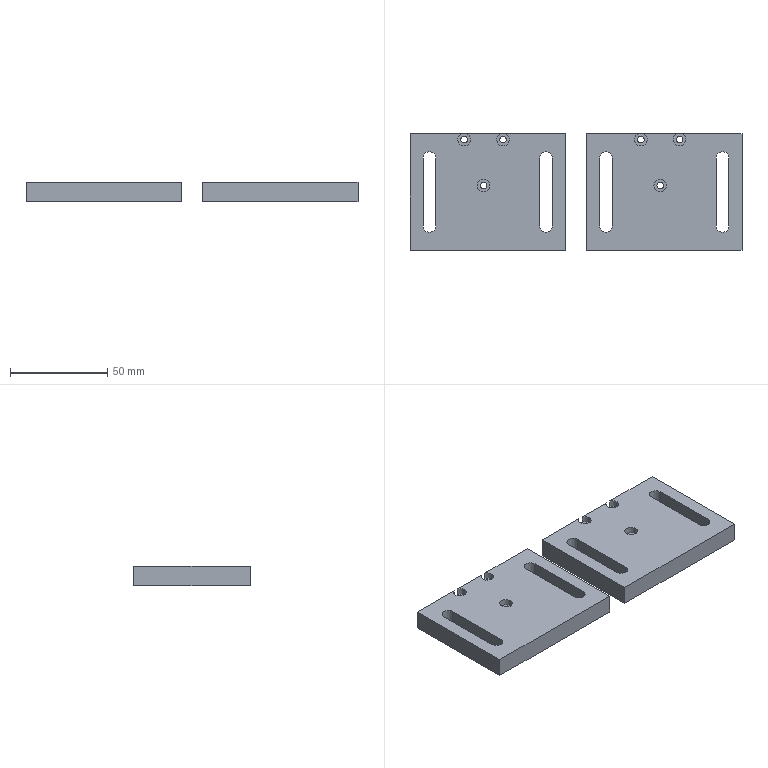Part | 2 solids | 46 faces | box 171 x 60 x 10 mm | volume 84542 mm3 | plane 26 | cylinder 20 | commonest cylinder face diameters 6.5 x14 3.4 x6
STEP:
#1=CARTESIAN_POINT('',(64.25,-17.5,0.));
#2=VERTEX_POINT('',#1);
#3=CARTESIAN_POINT('',(64.25,17.5,0.));
#4=VERTEX_POINT('',#3);
#5=CARTESIAN_POINT('',(64.25,-8.75,0.));
#6=DIRECTION('',(0.,1.,0.));
#7=VECTOR('',#6,1000.);
#8=LINE('',#5,#7);
#9=EDGE_CURVE('',#2,#4,#8,.T.);
#10=ORIENTED_EDGE('',*,*,#9,.T.);
#11=CARTESIAN_POINT('',(57.75,17.5,0.));
#12=VERTEX_POINT('',#11);
#13=CARTESIAN_POINT('',(61.,17.5,0.));
#14=DIRECTION('',(0.,0.,1.));
#15=DIRECTION('',(-1.,0.,0.));
#16=AXIS2_PLACEMENT_3D('',#13,#14,#15);
#17=CIRCLE('',#16,3.25);
#18=EDGE_CURVE('',#4,#12,#17,.T.);
#19=ORIENTED_EDGE('',*,*,#18,.T.);
#20=CARTESIAN_POINT('',(57.75,-17.5,0.));
#21=VERTEX_POINT('',#20);
#22=CARTESIAN_POINT('',(57.75,8.75,0.));
#23=DIRECTION('',(0.,-1.,0.));
#24=VECTOR('',#23,1000.);
#25=LINE('',#22,#24);
#26=EDGE_CURVE('',#12,#21,#25,.T.);
#27=ORIENTED_EDGE('',*,*,#26,.T.);
#28=CARTESIAN_POINT('',(61.,-17.5,0.));
#29=DIRECTION('',(0.,0.,1.));
#30=DIRECTION('',(1.,0.,0.));
#31=AXIS2_PLACEMENT_3D('',#28,#29,#30);
#32=CIRCLE('',#31,3.25);
#33=EDGE_CURVE('',#21,#2,#32,.T.);
#34=ORIENTED_EDGE('',*,*,#33,.T.);
#35=EDGE_LOOP('',(#10,#19,#27,#34));
#36=FACE_BOUND('',#35,.T.);
#37=CARTESIAN_POINT('',(124.25,-17.5,0.));
#38=VERTEX_POINT('',#37);
#39=CARTESIAN_POINT('',(124.25,17.5,0.));
#40=VERTEX_POINT('',#39);
#41=CARTESIAN_POINT('',(124.25,-8.75,0.));
#42=DIRECTION('',(0.,1.,0.));
#43=VECTOR('',#42,1000.);
#44=LINE('',#41,#43);
#45=EDGE_CURVE('',#38,#40,#44,.T.);
#46=ORIENTED_EDGE('',*,*,#45,.T.);
#47=CARTESIAN_POINT('',(117.75,17.5,0.));
#48=VERTEX_POINT('',#47);
#49=CARTESIAN_POINT('',(121.,17.5,0.));
#50=DIRECTION('',(0.,0.,1.));
#51=DIRECTION('',(-1.,0.,0.));
#52=AXIS2_PLACEMENT_3D('',#49,#50,#51);
#53=CIRCLE('',#52,3.25);
#54=EDGE_CURVE('',#40,#48,#53,.T.);
#55=ORIENTED_EDGE('',*,*,#54,.T.);
#56=CARTESIAN_POINT('',(117.75,-17.5,0.));
#57=VERTEX_POINT('',#56);
#58=CARTESIAN_POINT('',(117.75,8.75,0.));
#59=DIRECTION('',(0.,-1.,0.));
#60=VECTOR('',#59,1000.);
#61=LINE('',#58,#60);
#62=EDGE_CURVE('',#48,#57,#61,.T.);
#63=ORIENTED_EDGE('',*,*,#62,.T.);
#64=CARTESIAN_POINT('',(121.,-17.5,0.));
#65=DIRECTION('',(0.,0.,1.));
#66=DIRECTION('',(1.,0.,0.));
#67=AXIS2_PLACEMENT_3D('',#64,#65,#66);
#68=CIRCLE('',#67,3.25);
#69=EDGE_CURVE('',#57,#38,#68,.T.);
#70=ORIENTED_EDGE('',*,*,#69,.T.);
#71=EDGE_LOOP('',(#46,#55,#63,#70));
#72=FACE_BOUND('',#71,.T.);
#73=CARTESIAN_POINT('',(100.593,27.,0.));
#74=VERTEX_POINT('',#73);
#75=CARTESIAN_POINT('',(98.893,27.,0.));
#76=DIRECTION('',(0.,0.,1.));
#77=DIRECTION('',(1.,0.,0.));
#78=AXIS2_PLACEMENT_3D('',#75,#76,#77);
#79=CIRCLE('',#78,1.7);
#80=EDGE_CURVE('',#74,#74,#79,.T.);
#81=ORIENTED_EDGE('',*,*,#80,.T.);
#82=EDGE_LOOP('',(#81));
#83=FACE_BOUND('',#82,.T.);
#84=CARTESIAN_POINT('',(80.593,27.,0.));
#85=VERTEX_POINT('',#84);
#86=CARTESIAN_POINT('',(78.893,27.,0.));
#87=DIRECTION('',(0.,0.,1.));
#88=DIRECTION('',(1.,0.,0.));
#89=AXIS2_PLACEMENT_3D('',#86,#87,#88);
#90=CIRCLE('',#89,1.7);
#91=EDGE_CURVE('',#85,#85,#90,.T.);
#92=ORIENTED_EDGE('',*,*,#91,.T.);
#93=EDGE_LOOP('',(#92));
#94=FACE_BOUND('',#93,.T.);
#95=CARTESIAN_POINT('',(90.593,3.3,0.));
#96=VERTEX_POINT('',#95);
#97=CARTESIAN_POINT('',(88.893,3.3,0.));
#98=DIRECTION('',(0.,0.,1.));
#99=DIRECTION('',(1.,0.,0.));
#100=AXIS2_PLACEMENT_3D('',#97,#98,#99);
#101=CIRCLE('',#100,1.7);
#102=EDGE_CURVE('',#96,#96,#101,.T.);
#103=ORIENTED_EDGE('',*,*,#102,.T.);
#104=EDGE_LOOP('',(#103));
#105=FACE_BOUND('',#104,.T.);
#106=CARTESIAN_POINT('',(131.,-30.,0.));
#107=VERTEX_POINT('',#106);
#108=CARTESIAN_POINT('',(131.,30.,0.));
#109=VERTEX_POINT('',#108);
#110=CARTESIAN_POINT('',(131.,-30.,0.));
#111=DIRECTION('',(0.,1.,0.));
#112=VECTOR('',#111,1000.);
#113=LINE('',#110,#112);
#114=EDGE_CURVE('',#107,#109,#113,.T.);
#115=ORIENTED_EDGE('',*,*,#114,.F.);
#116=CARTESIAN_POINT('',(51.,-30.,0.));
#117=VERTEX_POINT('',#116);
#118=CARTESIAN_POINT('',(51.,-30.,0.));
#119=DIRECTION('',(1.,0.,0.));
#120=VECTOR('',#119,1000.);
#121=LINE('',#118,#120);
#122=EDGE_CURVE('',#117,#107,#121,.T.);
#123=ORIENTED_EDGE('',*,*,#122,.F.);
#124=CARTESIAN_POINT('',(51.,30.,0.));
#125=VERTEX_POINT('',#124);
#126=CARTESIAN_POINT('',(51.,30.,0.));
#127=DIRECTION('',(0.,-1.,0.));
#128=VECTOR('',#127,1000.);
#129=LINE('',#126,#128);
#130=EDGE_CURVE('',#125,#117,#129,.T.);
#131=ORIENTED_EDGE('',*,*,#130,.F.);
#132=CARTESIAN_POINT('',(131.,30.,0.));
#133=DIRECTION('',(-1.,0.,0.));
#134=VECTOR('',#133,1000.);
#135=LINE('',#132,#134);
#136=EDGE_CURVE('',#109,#125,#135,.T.);
#137=ORIENTED_EDGE('',*,*,#136,.F.);
#138=EDGE_LOOP('',(#115,#123,#131,#137));
#139=FACE_BOUND('',#138,.T.);
#140=CARTESIAN_POINT('',(91.,0.,0.));
#141=DIRECTION('',(0.,0.,1.));
#142=DIRECTION('',(1.,0.,0.));
#143=AXIS2_PLACEMENT_3D('',#140,#141,#142);
#144=PLANE('',#143);
#145=ADVANCED_FACE('',(#36,#72,#83,#94,#105,#139),#144,.F.);
#146=ORIENTED_EDGE('',*,*,#114,.T.);
#147=CARTESIAN_POINT('',(131.,30.,10.));
#148=VERTEX_POINT('',#147);
#149=CARTESIAN_POINT('',(131.,30.,0.));
#150=DIRECTION('',(0.,0.,1.));
#151=VECTOR('',#150,1000.);
#152=LINE('',#149,#151);
#153=EDGE_CURVE('',#109,#148,#152,.T.);
#154=ORIENTED_EDGE('',*,*,#153,.T.);
#155=CARTESIAN_POINT('',(131.,-30.,10.));
#156=VERTEX_POINT('',#155);
#157=CARTESIAN_POINT('',(131.,-30.,10.));
#158=DIRECTION('',(0.,1.,0.));
#159=VECTOR('',#158,1000.);
#160=LINE('',#157,#159);
#161=EDGE_CURVE('',#156,#148,#160,.T.);
#162=ORIENTED_EDGE('',*,*,#161,.F.);
#163=CARTESIAN_POINT('',(131.,-30.,0.));
#164=DIRECTION('',(0.,0.,1.));
#165=VECTOR('',#164,1000.);
#166=LINE('',#163,#165);
#167=EDGE_CURVE('',#107,#156,#166,.T.);
#168=ORIENTED_EDGE('',*,*,#167,.F.);
#169=EDGE_LOOP('',(#146,#154,#162,#168));
#170=FACE_BOUND('',#169,.T.);
#171=CARTESIAN_POINT('',(131.,-30.,0.));
#172=DIRECTION('',(1.,0.,0.));
#173=DIRECTION('',(0.,1.,0.));
#174=AXIS2_PLACEMENT_3D('',#171,#172,#173);
#175=PLANE('',#174);
#176=ADVANCED_FACE('',(#170),#175,.T.);
#177=CARTESIAN_POINT('',(80.143,30.,6.6));
#178=VERTEX_POINT('',#177);
#179=CARTESIAN_POINT('',(80.143,30.,10.));
#180=VERTEX_POINT('',#179);
#181=CARTESIAN_POINT('',(80.143,30.,8.3));
#182=DIRECTION('',(0.,0.,1.));
#183=VECTOR('',#182,1000.);
#184=LINE('',#181,#183);
#185=EDGE_CURVE('',#178,#180,#184,.T.);
#186=ORIENTED_EDGE('',*,*,#185,.T.);
#187=CARTESIAN_POINT('',(97.643,30.,10.));
#188=VERTEX_POINT('',#187);
#189=CARTESIAN_POINT('',(131.,30.,10.));
#190=DIRECTION('',(-1.,0.,0.));
#191=VECTOR('',#190,1000.);
#192=LINE('',#189,#191);
#193=EDGE_CURVE('',#188,#180,#192,.T.);
#194=ORIENTED_EDGE('',*,*,#193,.F.);
#195=CARTESIAN_POINT('',(97.643,30.,6.6));
#196=VERTEX_POINT('',#195);
#197=CARTESIAN_POINT('',(97.643,30.,8.3));
#198=DIRECTION('',(0.,0.,-1.));
#199=VECTOR('',#198,1000.);
#200=LINE('',#197,#199);
#201=EDGE_CURVE('',#188,#196,#200,.T.);
#202=ORIENTED_EDGE('',*,*,#201,.T.);
#203=CARTESIAN_POINT('',(100.143,30.,6.6));
#204=VERTEX_POINT('',#203);
#205=CARTESIAN_POINT('',(131.,30.,6.6));
#206=DIRECTION('',(1.,0.,0.));
#207=VECTOR('',#206,1000.);
#208=LINE('',#205,#207);
#209=EDGE_CURVE('',#196,#204,#208,.T.);
#210=ORIENTED_EDGE('',*,*,#209,.T.);
#211=CARTESIAN_POINT('',(100.143,30.,10.));
#212=VERTEX_POINT('',#211);
#213=CARTESIAN_POINT('',(100.143,30.,8.3));
#214=DIRECTION('',(0.,0.,1.));
#215=VECTOR('',#214,1000.);
#216=LINE('',#213,#215);
#217=EDGE_CURVE('',#204,#212,#216,.T.);
#218=ORIENTED_EDGE('',*,*,#217,.T.);
#219=CARTESIAN_POINT('',(131.,30.,10.));
#220=DIRECTION('',(-1.,0.,0.));
#221=VECTOR('',#220,1000.);
#222=LINE('',#219,#221);
#223=EDGE_CURVE('',#148,#212,#222,.T.);
#224=ORIENTED_EDGE('',*,*,#223,.F.);
#225=ORIENTED_EDGE('',*,*,#153,.F.);
#226=ORIENTED_EDGE('',*,*,#136,.T.);
#227=CARTESIAN_POINT('',(51.,30.,10.));
#228=VERTEX_POINT('',#227);
#229=CARTESIAN_POINT('',(51.,30.,0.));
#230=DIRECTION('',(0.,0.,1.));
#231=VECTOR('',#230,1000.);
#232=LINE('',#229,#231);
#233=EDGE_CURVE('',#125,#228,#232,.T.);
#234=ORIENTED_EDGE('',*,*,#233,.T.);
#235=CARTESIAN_POINT('',(77.643,30.,10.));
#236=VERTEX_POINT('',#235);
#237=CARTESIAN_POINT('',(131.,30.,10.));
#238=DIRECTION('',(-1.,0.,0.));
#239=VECTOR('',#238,1000.);
#240=LINE('',#237,#239);
#241=EDGE_CURVE('',#236,#228,#240,.T.);
#242=ORIENTED_EDGE('',*,*,#241,.F.);
#243=CARTESIAN_POINT('',(77.643,30.,6.6));
#244=VERTEX_POINT('',#243);
#245=CARTESIAN_POINT('',(77.643,30.,8.3));
#246=DIRECTION('',(0.,0.,-1.));
#247=VECTOR('',#246,1000.);
#248=LINE('',#245,#247);
#249=EDGE_CURVE('',#236,#244,#248,.T.);
#250=ORIENTED_EDGE('',*,*,#249,.T.);
#251=CARTESIAN_POINT('',(131.,30.,6.6));
#252=DIRECTION('',(1.,0.,0.));
#253=VECTOR('',#252,1000.);
#254=LINE('',#251,#253);
#255=EDGE_CURVE('',#244,#178,#254,.T.);
#256=ORIENTED_EDGE('',*,*,#255,.T.);
#257=EDGE_LOOP('',(#186,#194,#202,#210,#218,#224,#225,#226,#234,#242,#250,#256));
#258=FACE_BOUND('',#257,.T.);
#259=CARTESIAN_POINT('',(131.,30.,0.));
#260=DIRECTION('',(0.,1.,0.));
#261=DIRECTION('',(-1.,0.,0.));
#262=AXIS2_PLACEMENT_3D('',#259,#260,#261);
#263=PLANE('',#262);
#264=ADVANCED_FACE('',(#258),#263,.T.);
#265=ORIENTED_EDGE('',*,*,#130,.T.);
#266=CARTESIAN_POINT('',(51.,-30.,10.));
#267=VERTEX_POINT('',#266);
#268=CARTESIAN_POINT('',(51.,-30.,0.));
#269=DIRECTION('',(0.,0.,1.));
#270=VECTOR('',#269,1000.);
#271=LINE('',#268,#270);
#272=EDGE_CURVE('',#117,#267,#271,.T.);
#273=ORIENTED_EDGE('',*,*,#272,.T.);
#274=CARTESIAN_POINT('',(51.,30.,10.));
#275=DIRECTION('',(0.,-1.,0.));
#276=VECTOR('',#275,1000.);
#277=LINE('',#274,#276);
#278=EDGE_CURVE('',#228,#267,#277,.T.);
#279=ORIENTED_EDGE('',*,*,#278,.F.);
#280=ORIENTED_EDGE('',*,*,#233,.F.);
#281=EDGE_LOOP('',(#265,#273,#279,#280));
#282=FACE_BOUND('',#281,.T.);
#283=CARTESIAN_POINT('',(51.,30.,0.));
#284=DIRECTION('',(-1.,0.,0.));
#285=DIRECTION('',(0.,-1.,0.));
#286=AXIS2_PLACEMENT_3D('',#283,#284,#285);
#287=PLANE('',#286);
#288=ADVANCED_FACE('',(#282),#287,.T.);
#289=ORIENTED_EDGE('',*,*,#122,.T.);
#290=ORIENTED_EDGE('',*,*,#167,.T.);
#291=CARTESIAN_POINT('',(51.,-30.,10.));
#292=DIRECTION('',(1.,0.,0.));
#293=VECTOR('',#292,1000.);
#294=LINE('',#291,#293);
#295=EDGE_CURVE('',#267,#156,#294,.T.);
#296=ORIENTED_EDGE('',*,*,#295,.F.);
#297=ORIENTED_EDGE('',*,*,#272,.F.);
#298=EDGE_LOOP('',(#289,#290,#296,#297));
#299=FACE_BOUND('',#298,.T.);
#300=CARTESIAN_POINT('',(51.,-30.,0.));
#301=DIRECTION('',(0.,-1.,0.));
#302=DIRECTION('',(1.,0.,0.));
#303=AXIS2_PLACEMENT_3D('',#300,#301,#302);
#304=PLANE('',#303);
#305=ADVANCED_FACE('',(#299),#304,.T.);
#306=CARTESIAN_POINT('',(64.25,-17.5,10.));
#307=VERTEX_POINT('',#306);
#308=CARTESIAN_POINT('',(57.75,-17.5,10.));
#309=VERTEX_POINT('',#308);
#310=CARTESIAN_POINT('',(61.,-17.5,10.));
#311=DIRECTION('',(0.,0.,-1.));
#312=DIRECTION('',(1.,0.,0.));
#313=AXIS2_PLACEMENT_3D('',#310,#311,#312);
#314=CIRCLE('',#313,3.25);
#315=EDGE_CURVE('',#307,#309,#314,.T.);
#316=ORIENTED_EDGE('',*,*,#315,.F.);
#317=CARTESIAN_POINT('',(64.25,-17.5,0.));
#318=DIRECTION('',(0.,0.,1.));
#319=VECTOR('',#318,1000.);
#320=LINE('',#317,#319);
#321=EDGE_CURVE('',#2,#307,#320,.T.);
#322=ORIENTED_EDGE('',*,*,#321,.F.);
#323=ORIENTED_EDGE('',*,*,#33,.F.);
#324=CARTESIAN_POINT('',(57.75,-17.5,0.));
#325=DIRECTION('',(0.,0.,1.));
#326=VECTOR('',#325,1000.);
#327=LINE('',#324,#326);
#328=EDGE_CURVE('',#21,#309,#327,.T.);
#329=ORIENTED_EDGE('',*,*,#328,.T.);
#330=EDGE_LOOP('',(#316,#322,#323,#329));
#331=FACE_BOUND('',#330,.T.);
#332=CARTESIAN_POINT('',(61.,-17.5,0.));
#333=DIRECTION('',(0.,0.,1.));
#334=DIRECTION('',(1.,0.,0.));
#335=AXIS2_PLACEMENT_3D('',#332,#333,#334);
#336=CYLINDRICAL_SURFACE('',#335,3.25);
#337=ADVANCED_FACE('',(#331),#336,.F.);
#338=CARTESIAN_POINT('',(64.25,17.5,10.));
#339=VERTEX_POINT('',#338);
#340=CARTESIAN_POINT('',(64.25,-8.75,10.));
#341=DIRECTION('',(0.,-1.,0.));
#342=VECTOR('',#341,1000.);
#343=LINE('',#340,#342);
#344=EDGE_CURVE('',#339,#307,#343,.T.);
#345=ORIENTED_EDGE('',*,*,#344,.F.);
#346=CARTESIAN_POINT('',(64.25,17.5,0.));
#347=DIRECTION('',(0.,0.,1.));
#348=VECTOR('',#347,1000.);
#349=LINE('',#346,#348);
#350=EDGE_CURVE('',#4,#339,#349,.T.);
#351=ORIENTED_EDGE('',*,*,#350,.F.);
#352=ORIENTED_EDGE('',*,*,#9,.F.);
#353=ORIENTED_EDGE('',*,*,#321,.T.);
#354=EDGE_LOOP('',(#345,#351,#352,#353));
#355=FACE_BOUND('',#354,.T.);
#356=CARTESIAN_POINT('',(64.25,-17.5,0.));
#357=DIRECTION('',(1.,0.,0.));
#358=DIRECTION('',(0.,1.,0.));
#359=AXIS2_PLACEMENT_3D('',#356,#357,#358);
#360=PLANE('',#359);
#361=ADVANCED_FACE('',(#355),#360,.F.);
#362=CARTESIAN_POINT('',(57.75,17.5,10.));
#363=VERTEX_POINT('',#362);
#364=CARTESIAN_POINT('',(61.,17.5,10.));
#365=DIRECTION('',(0.,0.,-1.));
#366=DIRECTION('',(-1.,0.,0.));
#367=AXIS2_PLACEMENT_3D('',#364,#365,#366);
#368=CIRCLE('',#367,3.25);
#369=EDGE_CURVE('',#363,#339,#368,.T.);
#370=ORIENTED_EDGE('',*,*,#369,.F.);
#371=CARTESIAN_POINT('',(57.75,17.5,0.));
#372=DIRECTION('',(0.,0.,1.));
#373=VECTOR('',#372,1000.);
#374=LINE('',#371,#373);
#375=EDGE_CURVE('',#12,#363,#374,.T.);
#376=ORIENTED_EDGE('',*,*,#375,.F.);
#377=ORIENTED_EDGE('',*,*,#18,.F.);
#378=ORIENTED_EDGE('',*,*,#350,.T.);
#379=EDGE_LOOP('',(#370,#376,#377,#378));
#380=FACE_BOUND('',#379,.T.);
#381=CARTESIAN_POINT('',(61.,17.5,0.));
#382=DIRECTION('',(0.,0.,1.));
#383=DIRECTION('',(-1.,0.,0.));
#384=AXIS2_PLACEMENT_3D('',#381,#382,#383);
#385=CYLINDRICAL_SURFACE('',#384,3.25);
#386=ADVANCED_FACE('',(#380),#385,.F.);
#387=CARTESIAN_POINT('',(57.75,8.75,10.));
#388=DIRECTION('',(0.,1.,0.));
#389=VECTOR('',#388,1000.);
#390=LINE('',#387,#389);
#391=EDGE_CURVE('',#309,#363,#390,.T.);
#392=ORIENTED_EDGE('',*,*,#391,.F.);
#393=ORIENTED_EDGE('',*,*,#328,.F.);
#394=ORIENTED_EDGE('',*,*,#26,.F.);
#395=ORIENTED_EDGE('',*,*,#375,.T.);
#396=EDGE_LOOP('',(#392,#393,#394,#395));
#397=FACE_BOUND('',#396,.T.);
#398=CARTESIAN_POINT('',(57.75,17.5,0.));
#399=DIRECTION('',(-1.,0.,0.));
#400=DIRECTION('',(0.,-1.,0.));
#401=AXIS2_PLACEMENT_3D('',#398,#399,#400);
#402=PLANE('',#401);
#403=ADVANCED_FACE('',(#397),#402,.F.);
#404=CARTESIAN_POINT('',(124.25,-17.5,10.));
#405=VERTEX_POINT('',#404);
#406=CARTESIAN_POINT('',(117.75,-17.5,10.));
#407=VERTEX_POINT('',#406);
#408=CARTESIAN_POINT('',(121.,-17.5,10.));
#409=DIRECTION('',(0.,0.,-1.));
#410=DIRECTION('',(1.,0.,0.));
#411=AXIS2_PLACEMENT_3D('',#408,#409,#410);
#412=CIRCLE('',#411,3.25);
#413=EDGE_CURVE('',#405,#407,#412,.T.);
#414=ORIENTED_EDGE('',*,*,#413,.F.);
#415=CARTESIAN_POINT('',(124.25,-17.5,0.));
#416=DIRECTION('',(0.,0.,1.));
#417=VECTOR('',#416,1000.);
#418=LINE('',#415,#417);
#419=EDGE_CURVE('',#38,#405,#418,.T.);
#420=ORIENTED_EDGE('',*,*,#419,.F.);
#421=ORIENTED_EDGE('',*,*,#69,.F.);
#422=CARTESIAN_POINT('',(117.75,-17.5,0.));
#423=DIRECTION('',(0.,0.,1.));
#424=VECTOR('',#423,1000.);
#425=LINE('',#422,#424);
#426=EDGE_CURVE('',#57,#407,#425,.T.);
#427=ORIENTED_EDGE('',*,*,#426,.T.);
#428=EDGE_LOOP('',(#414,#420,#421,#427));
#429=FACE_BOUND('',#428,.T.);
#430=CARTESIAN_POINT('',(121.,-17.5,0.));
#431=DIRECTION('',(0.,0.,1.));
#432=DIRECTION('',(1.,0.,0.));
#433=AXIS2_PLACEMENT_3D('',#430,#431,#432);
#434=CYLINDRICAL_SURFACE('',#433,3.25);
#435=ADVANCED_FACE('',(#429),#434,.F.);
#436=CARTESIAN_POINT('',(124.25,17.5,10.));
#437=VERTEX_POINT('',#436);
#438=CARTESIAN_POINT('',(124.25,-8.75,10.));
#439=DIRECTION('',(0.,-1.,0.));
#440=VECTOR('',#439,1000.);
#441=LINE('',#438,#440);
#442=EDGE_CURVE('',#437,#405,#441,.T.);
#443=ORIENTED_EDGE('',*,*,#442,.F.);
#444=CARTESIAN_POINT('',(124.25,17.5,0.));
#445=DIRECTION('',(0.,0.,1.));
#446=VECTOR('',#445,1000.);
#447=LINE('',#444,#446);
#448=EDGE_CURVE('',#40,#437,#447,.T.);
#449=ORIENTED_EDGE('',*,*,#448,.F.);
#450=ORIENTED_EDGE('',*,*,#45,.F.);
#451=ORIENTED_EDGE('',*,*,#419,.T.);
#452=EDGE_LOOP('',(#443,#449,#450,#451));
#453=FACE_BOUND('',#452,.T.);
#454=CARTESIAN_POINT('',(124.25,-17.5,0.));
#455=DIRECTION('',(1.,0.,0.));
#456=DIRECTION('',(0.,1.,0.));
#457=AXIS2_PLACEMENT_3D('',#454,#455,#456);
#458=PLANE('',#457);
#459=ADVANCED_FACE('',(#453),#458,.F.);
#460=CARTESIAN_POINT('',(117.75,17.5,10.));
#461=VERTEX_POINT('',#460);
#462=CARTESIAN_POINT('',(121.,17.5,10.));
#463=DIRECTION('',(0.,0.,-1.));
#464=DIRECTION('',(-1.,0.,0.));
#465=AXIS2_PLACEMENT_3D('',#462,#463,#464);
#466=CIRCLE('',#465,3.25);
#467=EDGE_CURVE('',#461,#437,#466,.T.);
#468=ORIENTED_EDGE('',*,*,#467,.F.);
#469=CARTESIAN_POINT('',(117.75,17.5,0.));
#470=DIRECTION('',(0.,0.,1.));
#471=VECTOR('',#470,1000.);
#472=LINE('',#469,#471);
#473=EDGE_CURVE('',#48,#461,#472,.T.);
#474=ORIENTED_EDGE('',*,*,#473,.F.);
#475=ORIENTED_EDGE('',*,*,#54,.F.);
#476=ORIENTED_EDGE('',*,*,#448,.T.);
#477=EDGE_LOOP('',(#468,#474,#475,#476));
#478=FACE_BOUND('',#477,.T.);
#479=CARTESIAN_POINT('',(121.,17.5,0.));
#480=DIRECTION('',(0.,0.,1.));
#481=DIRECTION('',(-1.,0.,0.));
#482=AXIS2_PLACEMENT_3D('',#479,#480,#481);
#483=CYLINDRICAL_SURFACE('',#482,3.25);
#484=ADVANCED_FACE('',(#478),#483,.F.);
#485=CARTESIAN_POINT('',(117.75,8.75,10.));
#486=DIRECTION('',(0.,1.,0.));
#487=VECTOR('',#486,1000.);
#488=LINE('',#485,#487);
#489=EDGE_CURVE('',#407,#461,#488,.T.);
#490=ORIENTED_EDGE('',*,*,#489,.F.);
#491=ORIENTED_EDGE('',*,*,#426,.F.);
#492=ORIENTED_EDGE('',*,*,#62,.F.);
#493=ORIENTED_EDGE('',*,*,#473,.T.);
#494=EDGE_LOOP('',(#490,#491,#492,#493));
#495=FACE_BOUND('',#494,.T.);
#496=CARTESIAN_POINT('',(117.75,17.5,0.));
#497=DIRECTION('',(-1.,0.,0.));
#498=DIRECTION('',(0.,-1.,0.));
#499=AXIS2_PLACEMENT_3D('',#496,#497,#498);
#500=PLANE('',#499);
#501=ADVANCED_FACE('',(#495),#500,.F.);
#502=CARTESIAN_POINT('',(92.143,3.3,10.));
#503=VERTEX_POINT('',#502);
#504=CARTESIAN_POINT('',(88.893,3.3,10.));
#505=DIRECTION('',(0.,0.,-1.));
#506=DIRECTION('',(1.,0.,0.));
#507=AXIS2_PLACEMENT_3D('',#504,#505,#506);
#508=CIRCLE('',#507,3.25);
#509=EDGE_CURVE('',#503,#503,#508,.T.);
#510=ORIENTED_EDGE('',*,*,#509,.T.);
#511=EDGE_LOOP('',(#510));
#512=FACE_BOUND('',#511,.T.);
#513=ORIENTED_EDGE('',*,*,#442,.T.);
#514=ORIENTED_EDGE('',*,*,#413,.T.);
#515=ORIENTED_EDGE('',*,*,#489,.T.);
#516=ORIENTED_EDGE('',*,*,#467,.T.);
#517=EDGE_LOOP('',(#513,#514,#515,#516));
#518=FACE_BOUND('',#517,.T.);
#519=ORIENTED_EDGE('',*,*,#344,.T.);
#520=ORIENTED_EDGE('',*,*,#315,.T.);
#521=ORIENTED_EDGE('',*,*,#391,.T.);
#522=ORIENTED_EDGE('',*,*,#369,.T.);
#523=EDGE_LOOP('',(#519,#520,#521,#522));
#524=FACE_BOUND('',#523,.T.);
#525=CARTESIAN_POINT('',(78.893,27.,10.));
#526=DIRECTION('',(0.,0.,-1.));
#527=DIRECTION('',(1.,0.,0.));
#528=AXIS2_PLACEMENT_3D('',#525,#526,#527);
#529=CIRCLE('',#528,3.25);
#530=EDGE_CURVE('',#180,#236,#529,.T.);
#531=ORIENTED_EDGE('',*,*,#530,.T.);
#532=ORIENTED_EDGE('',*,*,#241,.T.);
#533=ORIENTED_EDGE('',*,*,#278,.T.);
#534=ORIENTED_EDGE('',*,*,#295,.T.);
#535=ORIENTED_EDGE('',*,*,#161,.T.);
#536=ORIENTED_EDGE('',*,*,#223,.T.);
#537=CARTESIAN_POINT('',(98.893,27.,10.));
#538=DIRECTION('',(0.,0.,-1.));
#539=DIRECTION('',(1.,0.,0.));
#540=AXIS2_PLACEMENT_3D('',#537,#538,#539);
#541=CIRCLE('',#540,3.25);
#542=EDGE_CURVE('',#212,#188,#541,.T.);
#543=ORIENTED_EDGE('',*,*,#542,.T.);
#544=ORIENTED_EDGE('',*,*,#193,.T.);
#545=EDGE_LOOP('',(#531,#532,#533,#534,#535,#536,#543,#544));
#546=FACE_BOUND('',#545,.T.);
#547=CARTESIAN_POINT('',(91.,0.,10.));
#548=DIRECTION('',(0.,0.,1.));
#549=DIRECTION('',(1.,0.,0.));
#550=AXIS2_PLACEMENT_3D('',#547,#548,#549);
#551=PLANE('',#550);
#552=ADVANCED_FACE('',(#512,#518,#524,#546),#551,.T.);
#553=ORIENTED_EDGE('',*,*,#80,.F.);
#554=EDGE_LOOP('',(#553));
#555=FACE_BOUND('',#554,.T.);
#556=CARTESIAN_POINT('',(100.593,27.,6.6));
#557=VERTEX_POINT('',#556);
#558=CARTESIAN_POINT('',(98.893,27.,6.6));
#559=DIRECTION('',(0.,0.,1.));
#560=DIRECTION('',(1.,0.,0.));
#561=AXIS2_PLACEMENT_3D('',#558,#559,#560);
#562=CIRCLE('',#561,1.7);
#563=EDGE_CURVE('',#557,#557,#562,.T.);
#564=ORIENTED_EDGE('',*,*,#563,.T.);
#565=EDGE_LOOP('',(#564));
#566=FACE_BOUND('',#565,.T.);
#567=CARTESIAN_POINT('',(98.893,27.,-90.499));
#568=DIRECTION('',(0.,0.,1.));
#569=DIRECTION('',(1.,0.,0.));
#570=AXIS2_PLACEMENT_3D('',#567,#568,#569);
#571=CYLINDRICAL_SURFACE('',#570,1.7);
#572=ADVANCED_FACE('',(#555,#566),#571,.F.);
#573=ORIENTED_EDGE('',*,*,#217,.F.);
#574=CARTESIAN_POINT('',(98.893,27.,6.6));
#575=DIRECTION('',(0.,0.,1.));
#576=DIRECTION('',(1.,0.,0.));
#577=AXIS2_PLACEMENT_3D('',#574,#575,#576);
#578=CIRCLE('',#577,3.25);
#579=EDGE_CURVE('',#196,#204,#578,.T.);
#580=ORIENTED_EDGE('',*,*,#579,.F.);
#581=ORIENTED_EDGE('',*,*,#201,.F.);
#582=ORIENTED_EDGE('',*,*,#542,.F.);
#583=EDGE_LOOP('',(#573,#580,#581,#582));
#584=FACE_BOUND('',#583,.T.);
#585=CARTESIAN_POINT('',(98.893,27.,8.3));
#586=DIRECTION('',(0.,0.,1.));
#587=DIRECTION('',(0.,-1.,0.));
#588=AXIS2_PLACEMENT_3D('',#585,#586,#587);
#589=CYLINDRICAL_SURFACE('',#588,3.25);
#590=ADVANCED_FACE('',(#584),#589,.F.);
#591=ORIENTED_EDGE('',*,*,#563,.F.);
#592=EDGE_LOOP('',(#591));
#593=FACE_BOUND('',#592,.T.);
#594=ORIENTED_EDGE('',*,*,#209,.F.);
#595=ORIENTED_EDGE('',*,*,#579,.T.);
#596=EDGE_LOOP('',(#594,#595));
#597=FACE_BOUND('',#596,.T.);
#598=CARTESIAN_POINT('',(88.893,3.3,6.6));
#599=DIRECTION('',(0.,0.,1.));
#600=DIRECTION('',(1.,0.,0.));
#601=AXIS2_PLACEMENT_3D('',#598,#599,#600);
#602=PLANE('',#601);
#603=ADVANCED_FACE('',(#593,#597),#602,.T.);
#604=ORIENTED_EDGE('',*,*,#91,.F.);
#605=EDGE_LOOP('',(#604));
#606=FACE_BOUND('',#605,.T.);
#607=CARTESIAN_POINT('',(80.593,27.,6.6));
#608=VERTEX_POINT('',#607);
#609=CARTESIAN_POINT('',(78.893,27.,6.6));
#610=DIRECTION('',(0.,0.,1.));
#611=DIRECTION('',(1.,0.,0.));
#612=AXIS2_PLACEMENT_3D('',#609,#610,#611);
#613=CIRCLE('',#612,1.7);
#614=EDGE_CURVE('',#608,#608,#613,.T.);
#615=ORIENTED_EDGE('',*,*,#614,.T.);
#616=EDGE_LOOP('',(#615));
#617=FACE_BOUND('',#616,.T.);
#618=CARTESIAN_POINT('',(78.893,27.,-90.499));
#619=DIRECTION('',(0.,0.,1.));
#620=DIRECTION('',(1.,0.,0.));
#621=AXIS2_PLACEMENT_3D('',#618,#619,#620);
#622=CYLINDRICAL_SURFACE('',#621,1.7);
#623=ADVANCED_FACE('',(#606,#617),#622,.F.);
#624=ORIENTED_EDGE('',*,*,#185,.F.);
#625=CARTESIAN_POINT('',(78.893,27.,6.6));
#626=DIRECTION('',(0.,0.,1.));
#627=DIRECTION('',(1.,0.,0.));
#628=AXIS2_PLACEMENT_3D('',#625,#626,#627);
#629=CIRCLE('',#628,3.25);
#630=EDGE_CURVE('',#244,#178,#629,.T.);
#631=ORIENTED_EDGE('',*,*,#630,.F.);
#632=ORIENTED_EDGE('',*,*,#249,.F.);
#633=ORIENTED_EDGE('',*,*,#530,.F.);
#634=EDGE_LOOP('',(#624,#631,#632,#633));
#635=FACE_BOUND('',#634,.T.);
#636=CARTESIAN_POINT('',(78.893,27.,8.3));
#637=DIRECTION('',(0.,0.,1.));
#638=DIRECTION('',(0.,-1.,0.));
#639=AXIS2_PLACEMENT_3D('',#636,#637,#638);
#640=CYLINDRICAL_SURFACE('',#639,3.25);
#641=ADVANCED_FACE('',(#635),#640,.F.);
#642=ORIENTED_EDGE('',*,*,#614,.F.);
#643=EDGE_LOOP('',(#642));
#644=FACE_BOUND('',#643,.T.);
#645=ORIENTED_EDGE('',*,*,#255,.F.);
#646=ORIENTED_EDGE('',*,*,#630,.T.);
#647=EDGE_LOOP('',(#645,#646));
#648=FACE_BOUND('',#647,.T.);
#649=CARTESIAN_POINT('',(88.893,3.3,6.6));
#650=DIRECTION('',(0.,0.,1.));
#651=DIRECTION('',(1.,0.,0.));
#652=AXIS2_PLACEMENT_3D('',#649,#650,#651);
#653=PLANE('',#652);
#654=ADVANCED_FACE('',(#644,#648),#653,.T.);
#655=ORIENTED_EDGE('',*,*,#102,.F.);
#656=EDGE_LOOP('',(#655));
#657=FACE_BOUND('',#656,.T.);
#658=CARTESIAN_POINT('',(90.593,3.3,6.6));
#659=VERTEX_POINT('',#658);
#660=CARTESIAN_POINT('',(88.893,3.3,6.6));
#661=DIRECTION('',(0.,0.,1.));
#662=DIRECTION('',(1.,0.,0.));
#663=AXIS2_PLACEMENT_3D('',#660,#661,#662);
#664=CIRCLE('',#663,1.7);
#665=EDGE_CURVE('',#659,#659,#664,.T.);
#666=ORIENTED_EDGE('',*,*,#665,.T.);
#667=EDGE_LOOP('',(#666));
#668=FACE_BOUND('',#667,.T.);
#669=CARTESIAN_POINT('',(88.893,3.3,-90.499));
#670=DIRECTION('',(0.,0.,1.));
#671=DIRECTION('',(1.,0.,0.));
#672=AXIS2_PLACEMENT_3D('',#669,#670,#671);
#673=CYLINDRICAL_SURFACE('',#672,1.7);
#674=ADVANCED_FACE('',(#657,#668),#673,.F.);
#675=CARTESIAN_POINT('',(92.143,3.3,6.6));
#676=VERTEX_POINT('',#675);
#677=CARTESIAN_POINT('',(88.893,3.3,6.6));
#678=DIRECTION('',(0.,0.,1.));
#679=DIRECTION('',(1.,0.,0.));
#680=AXIS2_PLACEMENT_3D('',#677,#678,#679);
#681=CIRCLE('',#680,3.25);
#682=EDGE_CURVE('',#676,#676,#681,.T.);
#683=ORIENTED_EDGE('',*,*,#682,.F.);
#684=EDGE_LOOP('',(#683));
#685=FACE_BOUND('',#684,.T.);
#686=ORIENTED_EDGE('',*,*,#509,.F.);
#687=EDGE_LOOP('',(#686));
#688=FACE_BOUND('',#687,.T.);
#689=CARTESIAN_POINT('',(88.893,3.3,8.3));
#690=DIRECTION('',(0.,0.,1.));
#691=DIRECTION('',(1.,0.,0.));
#692=AXIS2_PLACEMENT_3D('',#689,#690,#691);
#693=CYLINDRICAL_SURFACE('',#692,3.25);
#694=ADVANCED_FACE('',(#685,#688),#693,.F.);
#695=ORIENTED_EDGE('',*,*,#665,.F.);
#696=EDGE_LOOP('',(#695));
#697=FACE_BOUND('',#696,.T.);
#698=ORIENTED_EDGE('',*,*,#682,.T.);
#699=EDGE_LOOP('',(#698));
#700=FACE_BOUND('',#699,.T.);
#701=CARTESIAN_POINT('',(88.893,3.3,6.6));
#702=DIRECTION('',(0.,0.,1.));
#703=DIRECTION('',(1.,0.,0.));
#704=AXIS2_PLACEMENT_3D('',#701,#702,#703);
#705=PLANE('',#704);
#706=ADVANCED_FACE('',(#697,#700),#705,.T.);
#707=CLOSED_SHELL('',(#145,#176,#264,#288,#305,#337,#361,#386,#403,#435,#459,#484,#501,#552,#572,#590,#603,#623,#641,#654,#674,#694,#706));
#708=MANIFOLD_SOLID_BREP('',#707);
#709=CARTESIAN_POINT('',(-26.75,-17.5,0.));
#710=VERTEX_POINT('',#709);
#711=CARTESIAN_POINT('',(-26.75,17.5,0.));
#712=VERTEX_POINT('',#711);
#713=CARTESIAN_POINT('',(-26.75,-8.75,0.));
#714=DIRECTION('',(0.,1.,0.));
#715=VECTOR('',#714,1000.);
#716=LINE('',#713,#715);
#717=EDGE_CURVE('',#710,#712,#716,.T.);
#718=ORIENTED_EDGE('',*,*,#717,.T.);
#719=CARTESIAN_POINT('',(-33.25,17.5,0.));
#720=VERTEX_POINT('',#719);
#721=CARTESIAN_POINT('',(-30.,17.5,0.));
#722=DIRECTION('',(0.,0.,1.));
#723=DIRECTION('',(-1.,0.,0.));
#724=AXIS2_PLACEMENT_3D('',#721,#722,#723);
#725=CIRCLE('',#724,3.25);
#726=EDGE_CURVE('',#712,#720,#725,.T.);
#727=ORIENTED_EDGE('',*,*,#726,.T.);
#728=CARTESIAN_POINT('',(-33.25,-17.5,0.));
#729=VERTEX_POINT('',#728);
#730=CARTESIAN_POINT('',(-33.25,8.75,0.));
#731=DIRECTION('',(0.,-1.,0.));
#732=VECTOR('',#731,1000.);
#733=LINE('',#730,#732);
#734=EDGE_CURVE('',#720,#729,#733,.T.);
#735=ORIENTED_EDGE('',*,*,#734,.T.);
#736=CARTESIAN_POINT('',(-30.,-17.5,0.));
#737=DIRECTION('',(0.,0.,1.));
#738=DIRECTION('',(1.,0.,0.));
#739=AXIS2_PLACEMENT_3D('',#736,#737,#738);
#740=CIRCLE('',#739,3.25);
#741=EDGE_CURVE('',#729,#710,#740,.T.);
#742=ORIENTED_EDGE('',*,*,#741,.T.);
#743=EDGE_LOOP('',(#718,#727,#735,#742));
#744=FACE_BOUND('',#743,.T.);
#745=CARTESIAN_POINT('',(33.25,-17.5,0.));
#746=VERTEX_POINT('',#745);
#747=CARTESIAN_POINT('',(33.25,17.5,0.));
#748=VERTEX_POINT('',#747);
#749=CARTESIAN_POINT('',(33.25,-8.75,0.));
#750=DIRECTION('',(0.,1.,0.));
#751=VECTOR('',#750,1000.);
#752=LINE('',#749,#751);
#753=EDGE_CURVE('',#746,#748,#752,.T.);
#754=ORIENTED_EDGE('',*,*,#753,.T.);
#755=CARTESIAN_POINT('',(26.75,17.5,0.));
#756=VERTEX_POINT('',#755);
#757=CARTESIAN_POINT('',(30.,17.5,0.));
#758=DIRECTION('',(0.,0.,1.));
#759=DIRECTION('',(-1.,0.,0.));
#760=AXIS2_PLACEMENT_3D('',#757,#758,#759);
#761=CIRCLE('',#760,3.25);
#762=EDGE_CURVE('',#748,#756,#761,.T.);
#763=ORIENTED_EDGE('',*,*,#762,.T.);
#764=CARTESIAN_POINT('',(26.75,-17.5,0.));
#765=VERTEX_POINT('',#764);
#766=CARTESIAN_POINT('',(26.75,8.75,0.));
#767=DIRECTION('',(0.,-1.,0.));
#768=VECTOR('',#767,1000.);
#769=LINE('',#766,#768);
#770=EDGE_CURVE('',#756,#765,#769,.T.);
#771=ORIENTED_EDGE('',*,*,#770,.T.);
#772=CARTESIAN_POINT('',(30.,-17.5,0.));
#773=DIRECTION('',(0.,0.,1.));
#774=DIRECTION('',(1.,0.,0.));
#775=AXIS2_PLACEMENT_3D('',#772,#773,#774);
#776=CIRCLE('',#775,3.25);
#777=EDGE_CURVE('',#765,#746,#776,.T.);
#778=ORIENTED_EDGE('',*,*,#777,.T.);
#779=EDGE_LOOP('',(#754,#763,#771,#778));
#780=FACE_BOUND('',#779,.T.);
#781=CARTESIAN_POINT('',(9.593,27.,0.));
#782=VERTEX_POINT('',#781);
#783=CARTESIAN_POINT('',(7.893,27.,0.));
#784=DIRECTION('',(0.,0.,1.));
#785=DIRECTION('',(1.,0.,0.));
#786=AXIS2_PLACEMENT_3D('',#783,#784,#785);
#787=CIRCLE('',#786,1.7);
#788=EDGE_CURVE('',#782,#782,#787,.T.);
#789=ORIENTED_EDGE('',*,*,#788,.T.);
#790=EDGE_LOOP('',(#789));
#791=FACE_BOUND('',#790,.T.);
#792=CARTESIAN_POINT('',(-10.407,27.,0.));
#793=VERTEX_POINT('',#792);
#794=CARTESIAN_POINT('',(-12.107,27.,0.));
#795=DIRECTION('',(0.,0.,1.));
#796=DIRECTION('',(1.,0.,0.));
#797=AXIS2_PLACEMENT_3D('',#794,#795,#796);
#798=CIRCLE('',#797,1.7);
#799=EDGE_CURVE('',#793,#793,#798,.T.);
#800=ORIENTED_EDGE('',*,*,#799,.T.);
#801=EDGE_LOOP('',(#800));
#802=FACE_BOUND('',#801,.T.);
#803=CARTESIAN_POINT('',(-0.4065,3.3,0.));
#804=VERTEX_POINT('',#803);
#805=CARTESIAN_POINT('',(-2.107,3.3,0.));
#806=DIRECTION('',(0.,0.,1.));
#807=DIRECTION('',(1.,0.,0.));
#808=AXIS2_PLACEMENT_3D('',#805,#806,#807);
#809=CIRCLE('',#808,1.7);
#810=EDGE_CURVE('',#804,#804,#809,.T.);
#811=ORIENTED_EDGE('',*,*,#810,.T.);
#812=EDGE_LOOP('',(#811));
#813=FACE_BOUND('',#812,.T.);
#814=CARTESIAN_POINT('',(40.,-30.,0.));
#815=VERTEX_POINT('',#814);
#816=CARTESIAN_POINT('',(40.,30.,0.));
#817=VERTEX_POINT('',#816);
#818=CARTESIAN_POINT('',(40.,-30.,0.));
#819=DIRECTION('',(0.,1.,0.));
#820=VECTOR('',#819,1000.);
#821=LINE('',#818,#820);
#822=EDGE_CURVE('',#815,#817,#821,.T.);
#823=ORIENTED_EDGE('',*,*,#822,.F.);
#824=CARTESIAN_POINT('',(-40.,-30.,0.));
#825=VERTEX_POINT('',#824);
#826=CARTESIAN_POINT('',(-40.,-30.,0.));
#827=DIRECTION('',(1.,0.,0.));
#828=VECTOR('',#827,1000.);
#829=LINE('',#826,#828);
#830=EDGE_CURVE('',#825,#815,#829,.T.);
#831=ORIENTED_EDGE('',*,*,#830,.F.);
#832=CARTESIAN_POINT('',(-40.,30.,0.));
#833=VERTEX_POINT('',#832);
#834=CARTESIAN_POINT('',(-40.,30.,0.));
#835=DIRECTION('',(0.,-1.,0.));
#836=VECTOR('',#835,1000.);
#837=LINE('',#834,#836);
#838=EDGE_CURVE('',#833,#825,#837,.T.);
#839=ORIENTED_EDGE('',*,*,#838,.F.);
#840=CARTESIAN_POINT('',(40.,30.,0.));
#841=DIRECTION('',(-1.,0.,0.));
#842=VECTOR('',#841,1000.);
#843=LINE('',#840,#842);
#844=EDGE_CURVE('',#817,#833,#843,.T.);
#845=ORIENTED_EDGE('',*,*,#844,.F.);
#846=EDGE_LOOP('',(#823,#831,#839,#845));
#847=FACE_BOUND('',#846,.T.);
#848=CARTESIAN_POINT('',(0.,0.,0.));
#849=DIRECTION('',(0.,0.,1.));
#850=DIRECTION('',(1.,0.,0.));
#851=AXIS2_PLACEMENT_3D('',#848,#849,#850);
#852=PLANE('',#851);
#853=ADVANCED_FACE('',(#744,#780,#791,#802,#813,#847),#852,.F.);
#854=ORIENTED_EDGE('',*,*,#822,.T.);
#855=CARTESIAN_POINT('',(40.,30.,10.));
#856=VERTEX_POINT('',#855);
#857=CARTESIAN_POINT('',(40.,30.,0.));
#858=DIRECTION('',(0.,0.,1.));
#859=VECTOR('',#858,1000.);
#860=LINE('',#857,#859);
#861=EDGE_CURVE('',#817,#856,#860,.T.);
#862=ORIENTED_EDGE('',*,*,#861,.T.);
#863=CARTESIAN_POINT('',(40.,-30.,10.));
#864=VERTEX_POINT('',#863);
#865=CARTESIAN_POINT('',(40.,-30.,10.));
#866=DIRECTION('',(0.,1.,0.));
#867=VECTOR('',#866,1000.);
#868=LINE('',#865,#867);
#869=EDGE_CURVE('',#864,#856,#868,.T.);
#870=ORIENTED_EDGE('',*,*,#869,.F.);
#871=CARTESIAN_POINT('',(40.,-30.,0.));
#872=DIRECTION('',(0.,0.,1.));
#873=VECTOR('',#872,1000.);
#874=LINE('',#871,#873);
#875=EDGE_CURVE('',#815,#864,#874,.T.);
#876=ORIENTED_EDGE('',*,*,#875,.F.);
#877=EDGE_LOOP('',(#854,#862,#870,#876));
#878=FACE_BOUND('',#877,.T.);
#879=CARTESIAN_POINT('',(40.,-30.,0.));
#880=DIRECTION('',(1.,0.,0.));
#881=DIRECTION('',(0.,1.,0.));
#882=AXIS2_PLACEMENT_3D('',#879,#880,#881);
#883=PLANE('',#882);
#884=ADVANCED_FACE('',(#878),#883,.T.);
#885=CARTESIAN_POINT('',(-10.857,30.,6.6));
#886=VERTEX_POINT('',#885);
#887=CARTESIAN_POINT('',(-10.857,30.,10.));
#888=VERTEX_POINT('',#887);
#889=CARTESIAN_POINT('',(-10.857,30.,8.3));
#890=DIRECTION('',(0.,0.,1.));
#891=VECTOR('',#890,1000.);
#892=LINE('',#889,#891);
#893=EDGE_CURVE('',#886,#888,#892,.T.);
#894=ORIENTED_EDGE('',*,*,#893,.T.);
#895=CARTESIAN_POINT('',(6.643,30.,10.));
#896=VERTEX_POINT('',#895);
#897=CARTESIAN_POINT('',(40.,30.,10.));
#898=DIRECTION('',(-1.,0.,0.));
#899=VECTOR('',#898,1000.);
#900=LINE('',#897,#899);
#901=EDGE_CURVE('',#896,#888,#900,.T.);
#902=ORIENTED_EDGE('',*,*,#901,.F.);
#903=CARTESIAN_POINT('',(6.643,30.,6.6));
#904=VERTEX_POINT('',#903);
#905=CARTESIAN_POINT('',(6.643,30.,8.3));
#906=DIRECTION('',(0.,0.,-1.));
#907=VECTOR('',#906,1000.);
#908=LINE('',#905,#907);
#909=EDGE_CURVE('',#896,#904,#908,.T.);
#910=ORIENTED_EDGE('',*,*,#909,.T.);
#911=CARTESIAN_POINT('',(9.143,30.,6.6));
#912=VERTEX_POINT('',#911);
#913=CARTESIAN_POINT('',(40.,30.,6.6));
#914=DIRECTION('',(1.,0.,0.));
#915=VECTOR('',#914,1000.);
#916=LINE('',#913,#915);
#917=EDGE_CURVE('',#904,#912,#916,.T.);
#918=ORIENTED_EDGE('',*,*,#917,.T.);
#919=CARTESIAN_POINT('',(9.143,30.,10.));
#920=VERTEX_POINT('',#919);
#921=CARTESIAN_POINT('',(9.143,30.,8.3));
#922=DIRECTION('',(0.,0.,1.));
#923=VECTOR('',#922,1000.);
#924=LINE('',#921,#923);
#925=EDGE_CURVE('',#912,#920,#924,.T.);
#926=ORIENTED_EDGE('',*,*,#925,.T.);
#927=CARTESIAN_POINT('',(40.,30.,10.));
#928=DIRECTION('',(-1.,0.,0.));
#929=VECTOR('',#928,1000.);
#930=LINE('',#927,#929);
#931=EDGE_CURVE('',#856,#920,#930,.T.);
#932=ORIENTED_EDGE('',*,*,#931,.F.);
#933=ORIENTED_EDGE('',*,*,#861,.F.);
#934=ORIENTED_EDGE('',*,*,#844,.T.);
#935=CARTESIAN_POINT('',(-40.,30.,10.));
#936=VERTEX_POINT('',#935);
#937=CARTESIAN_POINT('',(-40.,30.,0.));
#938=DIRECTION('',(0.,0.,1.));
#939=VECTOR('',#938,1000.);
#940=LINE('',#937,#939);
#941=EDGE_CURVE('',#833,#936,#940,.T.);
#942=ORIENTED_EDGE('',*,*,#941,.T.);
#943=CARTESIAN_POINT('',(-13.357,30.,10.));
#944=VERTEX_POINT('',#943);
#945=CARTESIAN_POINT('',(40.,30.,10.));
#946=DIRECTION('',(-1.,0.,0.));
#947=VECTOR('',#946,1000.);
#948=LINE('',#945,#947);
#949=EDGE_CURVE('',#944,#936,#948,.T.);
#950=ORIENTED_EDGE('',*,*,#949,.F.);
#951=CARTESIAN_POINT('',(-13.357,30.,6.6));
#952=VERTEX_POINT('',#951);
#953=CARTESIAN_POINT('',(-13.357,30.,8.3));
#954=DIRECTION('',(0.,0.,-1.));
#955=VECTOR('',#954,1000.);
#956=LINE('',#953,#955);
#957=EDGE_CURVE('',#944,#952,#956,.T.);
#958=ORIENTED_EDGE('',*,*,#957,.T.);
#959=CARTESIAN_POINT('',(40.,30.,6.6));
#960=DIRECTION('',(1.,0.,0.));
#961=VECTOR('',#960,1000.);
#962=LINE('',#959,#961);
#963=EDGE_CURVE('',#952,#886,#962,.T.);
#964=ORIENTED_EDGE('',*,*,#963,.T.);
#965=EDGE_LOOP('',(#894,#902,#910,#918,#926,#932,#933,#934,#942,#950,#958,#964));
#966=FACE_BOUND('',#965,.T.);
#967=CARTESIAN_POINT('',(40.,30.,0.));
#968=DIRECTION('',(0.,1.,0.));
#969=DIRECTION('',(-1.,0.,0.));
#970=AXIS2_PLACEMENT_3D('',#967,#968,#969);
#971=PLANE('',#970);
#972=ADVANCED_FACE('',(#966),#971,.T.);
#973=ORIENTED_EDGE('',*,*,#838,.T.);
#974=CARTESIAN_POINT('',(-40.,-30.,10.));
#975=VERTEX_POINT('',#974);
#976=CARTESIAN_POINT('',(-40.,-30.,0.));
#977=DIRECTION('',(0.,0.,1.));
#978=VECTOR('',#977,1000.);
#979=LINE('',#976,#978);
#980=EDGE_CURVE('',#825,#975,#979,.T.);
#981=ORIENTED_EDGE('',*,*,#980,.T.);
#982=CARTESIAN_POINT('',(-40.,30.,10.));
#983=DIRECTION('',(0.,-1.,0.));
#984=VECTOR('',#983,1000.);
#985=LINE('',#982,#984);
#986=EDGE_CURVE('',#936,#975,#985,.T.);
#987=ORIENTED_EDGE('',*,*,#986,.F.);
#988=ORIENTED_EDGE('',*,*,#941,.F.);
#989=EDGE_LOOP('',(#973,#981,#987,#988));
#990=FACE_BOUND('',#989,.T.);
#991=CARTESIAN_POINT('',(-40.,30.,0.));
#992=DIRECTION('',(-1.,0.,0.));
#993=DIRECTION('',(0.,-1.,0.));
#994=AXIS2_PLACEMENT_3D('',#991,#992,#993);
#995=PLANE('',#994);
#996=ADVANCED_FACE('',(#990),#995,.T.);
#997=ORIENTED_EDGE('',*,*,#830,.T.);
#998=ORIENTED_EDGE('',*,*,#875,.T.);
#999=CARTESIAN_POINT('',(-40.,-30.,10.));
#1000=DIRECTION('',(1.,0.,0.));
#1001=VECTOR('',#1000,1000.);
#1002=LINE('',#999,#1001);
#1003=EDGE_CURVE('',#975,#864,#1002,.T.);
#1004=ORIENTED_EDGE('',*,*,#1003,.F.);
#1005=ORIENTED_EDGE('',*,*,#980,.F.);
#1006=EDGE_LOOP('',(#997,#998,#1004,#1005));
#1007=FACE_BOUND('',#1006,.T.);
#1008=CARTESIAN_POINT('',(-40.,-30.,0.));
#1009=DIRECTION('',(0.,-1.,0.));
#1010=DIRECTION('',(1.,0.,0.));
#1011=AXIS2_PLACEMENT_3D('',#1008,#1009,#1010);
#1012=PLANE('',#1011);
#1013=ADVANCED_FACE('',(#1007),#1012,.T.);
#1014=CARTESIAN_POINT('',(-26.75,-17.5,10.));
#1015=VERTEX_POINT('',#1014);
#1016=CARTESIAN_POINT('',(-33.25,-17.5,10.));
#1017=VERTEX_POINT('',#1016);
#1018=CARTESIAN_POINT('',(-30.,-17.5,10.));
#1019=DIRECTION('',(0.,0.,-1.));
#1020=DIRECTION('',(1.,0.,0.));
#1021=AXIS2_PLACEMENT_3D('',#1018,#1019,#1020);
#1022=CIRCLE('',#1021,3.25);
#1023=EDGE_CURVE('',#1015,#1017,#1022,.T.);
#1024=ORIENTED_EDGE('',*,*,#1023,.F.);
#1025=CARTESIAN_POINT('',(-26.75,-17.5,0.));
#1026=DIRECTION('',(0.,0.,1.));
#1027=VECTOR('',#1026,1000.);
#1028=LINE('',#1025,#1027);
#1029=EDGE_CURVE('',#710,#1015,#1028,.T.);
#1030=ORIENTED_EDGE('',*,*,#1029,.F.);
#1031=ORIENTED_EDGE('',*,*,#741,.F.);
#1032=CARTESIAN_POINT('',(-33.25,-17.5,0.));
#1033=DIRECTION('',(0.,0.,1.));
#1034=VECTOR('',#1033,1000.);
#1035=LINE('',#1032,#1034);
#1036=EDGE_CURVE('',#729,#1017,#1035,.T.);
#1037=ORIENTED_EDGE('',*,*,#1036,.T.);
#1038=EDGE_LOOP('',(#1024,#1030,#1031,#1037));
#1039=FACE_BOUND('',#1038,.T.);
#1040=CARTESIAN_POINT('',(-30.,-17.5,0.));
#1041=DIRECTION('',(0.,0.,1.));
#1042=DIRECTION('',(1.,0.,0.));
#1043=AXIS2_PLACEMENT_3D('',#1040,#1041,#1042);
#1044=CYLINDRICAL_SURFACE('',#1043,3.25);
#1045=ADVANCED_FACE('',(#1039),#1044,.F.);
#1046=CARTESIAN_POINT('',(-26.75,17.5,10.));
#1047=VERTEX_POINT('',#1046);
#1048=CARTESIAN_POINT('',(-26.75,-8.75,10.));
#1049=DIRECTION('',(0.,-1.,0.));
#1050=VECTOR('',#1049,1000.);
#1051=LINE('',#1048,#1050);
#1052=EDGE_CURVE('',#1047,#1015,#1051,.T.);
#1053=ORIENTED_EDGE('',*,*,#1052,.F.);
#1054=CARTESIAN_POINT('',(-26.75,17.5,0.));
#1055=DIRECTION('',(0.,0.,1.));
#1056=VECTOR('',#1055,1000.);
#1057=LINE('',#1054,#1056);
#1058=EDGE_CURVE('',#712,#1047,#1057,.T.);
#1059=ORIENTED_EDGE('',*,*,#1058,.F.);
#1060=ORIENTED_EDGE('',*,*,#717,.F.);
#1061=ORIENTED_EDGE('',*,*,#1029,.T.);
#1062=EDGE_LOOP('',(#1053,#1059,#1060,#1061));
#1063=FACE_BOUND('',#1062,.T.);
#1064=CARTESIAN_POINT('',(-26.75,-17.5,0.));
#1065=DIRECTION('',(1.,0.,0.));
#1066=DIRECTION('',(0.,1.,0.));
#1067=AXIS2_PLACEMENT_3D('',#1064,#1065,#1066);
#1068=PLANE('',#1067);
#1069=ADVANCED_FACE('',(#1063),#1068,.F.);
#1070=CARTESIAN_POINT('',(-33.25,17.5,10.));
#1071=VERTEX_POINT('',#1070);
#1072=CARTESIAN_POINT('',(-30.,17.5,10.));
#1073=DIRECTION('',(0.,0.,-1.));
#1074=DIRECTION('',(-1.,0.,0.));
#1075=AXIS2_PLACEMENT_3D('',#1072,#1073,#1074);
#1076=CIRCLE('',#1075,3.25);
#1077=EDGE_CURVE('',#1071,#1047,#1076,.T.);
#1078=ORIENTED_EDGE('',*,*,#1077,.F.);
#1079=CARTESIAN_POINT('',(-33.25,17.5,0.));
#1080=DIRECTION('',(0.,0.,1.));
#1081=VECTOR('',#1080,1000.);
#1082=LINE('',#1079,#1081);
#1083=EDGE_CURVE('',#720,#1071,#1082,.T.);
#1084=ORIENTED_EDGE('',*,*,#1083,.F.);
#1085=ORIENTED_EDGE('',*,*,#726,.F.);
#1086=ORIENTED_EDGE('',*,*,#1058,.T.);
#1087=EDGE_LOOP('',(#1078,#1084,#1085,#1086));
#1088=FACE_BOUND('',#1087,.T.);
#1089=CARTESIAN_POINT('',(-30.,17.5,0.));
#1090=DIRECTION('',(0.,0.,1.));
#1091=DIRECTION('',(-1.,0.,0.));
#1092=AXIS2_PLACEMENT_3D('',#1089,#1090,#1091);
#1093=CYLINDRICAL_SURFACE('',#1092,3.25);
#1094=ADVANCED_FACE('',(#1088),#1093,.F.);
#1095=CARTESIAN_POINT('',(-33.25,8.75,10.));
#1096=DIRECTION('',(0.,1.,0.));
#1097=VECTOR('',#1096,1000.);
#1098=LINE('',#1095,#1097);
#1099=EDGE_CURVE('',#1017,#1071,#1098,.T.);
#1100=ORIENTED_EDGE('',*,*,#1099,.F.);
#1101=ORIENTED_EDGE('',*,*,#1036,.F.);
#1102=ORIENTED_EDGE('',*,*,#734,.F.);
#1103=ORIENTED_EDGE('',*,*,#1083,.T.);
#1104=EDGE_LOOP('',(#1100,#1101,#1102,#1103));
#1105=FACE_BOUND('',#1104,.T.);
#1106=CARTESIAN_POINT('',(-33.25,17.5,0.));
#1107=DIRECTION('',(-1.,0.,0.));
#1108=DIRECTION('',(0.,-1.,0.));
#1109=AXIS2_PLACEMENT_3D('',#1106,#1107,#1108);
#1110=PLANE('',#1109);
#1111=ADVANCED_FACE('',(#1105),#1110,.F.);
#1112=CARTESIAN_POINT('',(33.25,-17.5,10.));
#1113=VERTEX_POINT('',#1112);
#1114=CARTESIAN_POINT('',(26.75,-17.5,10.));
#1115=VERTEX_POINT('',#1114);
#1116=CARTESIAN_POINT('',(30.,-17.5,10.));
#1117=DIRECTION('',(0.,0.,-1.));
#1118=DIRECTION('',(1.,0.,0.));
#1119=AXIS2_PLACEMENT_3D('',#1116,#1117,#1118);
#1120=CIRCLE('',#1119,3.25);
#1121=EDGE_CURVE('',#1113,#1115,#1120,.T.);
#1122=ORIENTED_EDGE('',*,*,#1121,.F.);
#1123=CARTESIAN_POINT('',(33.25,-17.5,0.));
#1124=DIRECTION('',(0.,0.,1.));
#1125=VECTOR('',#1124,1000.);
#1126=LINE('',#1123,#1125);
#1127=EDGE_CURVE('',#746,#1113,#1126,.T.);
#1128=ORIENTED_EDGE('',*,*,#1127,.F.);
#1129=ORIENTED_EDGE('',*,*,#777,.F.);
#1130=CARTESIAN_POINT('',(26.75,-17.5,0.));
#1131=DIRECTION('',(0.,0.,1.));
#1132=VECTOR('',#1131,1000.);
#1133=LINE('',#1130,#1132);
#1134=EDGE_CURVE('',#765,#1115,#1133,.T.);
#1135=ORIENTED_EDGE('',*,*,#1134,.T.);
#1136=EDGE_LOOP('',(#1122,#1128,#1129,#1135));
#1137=FACE_BOUND('',#1136,.T.);
#1138=CARTESIAN_POINT('',(30.,-17.5,0.));
#1139=DIRECTION('',(0.,0.,1.));
#1140=DIRECTION('',(1.,0.,0.));
#1141=AXIS2_PLACEMENT_3D('',#1138,#1139,#1140);
#1142=CYLINDRICAL_SURFACE('',#1141,3.25);
#1143=ADVANCED_FACE('',(#1137),#1142,.F.);
#1144=CARTESIAN_POINT('',(33.25,17.5,10.));
#1145=VERTEX_POINT('',#1144);
#1146=CARTESIAN_POINT('',(33.25,-8.75,10.));
#1147=DIRECTION('',(0.,-1.,0.));
#1148=VECTOR('',#1147,1000.);
#1149=LINE('',#1146,#1148);
#1150=EDGE_CURVE('',#1145,#1113,#1149,.T.);
#1151=ORIENTED_EDGE('',*,*,#1150,.F.);
#1152=CARTESIAN_POINT('',(33.25,17.5,0.));
#1153=DIRECTION('',(0.,0.,1.));
#1154=VECTOR('',#1153,1000.);
#1155=LINE('',#1152,#1154);
#1156=EDGE_CURVE('',#748,#1145,#1155,.T.);
#1157=ORIENTED_EDGE('',*,*,#1156,.F.);
#1158=ORIENTED_EDGE('',*,*,#753,.F.);
#1159=ORIENTED_EDGE('',*,*,#1127,.T.);
#1160=EDGE_LOOP('',(#1151,#1157,#1158,#1159));
#1161=FACE_BOUND('',#1160,.T.);
#1162=CARTESIAN_POINT('',(33.25,-17.5,0.));
#1163=DIRECTION('',(1.,0.,0.));
#1164=DIRECTION('',(0.,1.,0.));
#1165=AXIS2_PLACEMENT_3D('',#1162,#1163,#1164);
#1166=PLANE('',#1165);
#1167=ADVANCED_FACE('',(#1161),#1166,.F.);
#1168=CARTESIAN_POINT('',(26.75,17.5,10.));
#1169=VERTEX_POINT('',#1168);
#1170=CARTESIAN_POINT('',(30.,17.5,10.));
#1171=DIRECTION('',(0.,0.,-1.));
#1172=DIRECTION('',(-1.,0.,0.));
#1173=AXIS2_PLACEMENT_3D('',#1170,#1171,#1172);
#1174=CIRCLE('',#1173,3.25);
#1175=EDGE_CURVE('',#1169,#1145,#1174,.T.);
#1176=ORIENTED_EDGE('',*,*,#1175,.F.);
#1177=CARTESIAN_POINT('',(26.75,17.5,0.));
#1178=DIRECTION('',(0.,0.,1.));
#1179=VECTOR('',#1178,1000.);
#1180=LINE('',#1177,#1179);
#1181=EDGE_CURVE('',#756,#1169,#1180,.T.);
#1182=ORIENTED_EDGE('',*,*,#1181,.F.);
#1183=ORIENTED_EDGE('',*,*,#762,.F.);
#1184=ORIENTED_EDGE('',*,*,#1156,.T.);
#1185=EDGE_LOOP('',(#1176,#1182,#1183,#1184));
#1186=FACE_BOUND('',#1185,.T.);
#1187=CARTESIAN_POINT('',(30.,17.5,0.));
#1188=DIRECTION('',(0.,0.,1.));
#1189=DIRECTION('',(-1.,0.,0.));
#1190=AXIS2_PLACEMENT_3D('',#1187,#1188,#1189);
#1191=CYLINDRICAL_SURFACE('',#1190,3.25);
#1192=ADVANCED_FACE('',(#1186),#1191,.F.);
#1193=CARTESIAN_POINT('',(26.75,8.75,10.));
#1194=DIRECTION('',(0.,1.,0.));
#1195=VECTOR('',#1194,1000.);
#1196=LINE('',#1193,#1195);
#1197=EDGE_CURVE('',#1115,#1169,#1196,.T.);
#1198=ORIENTED_EDGE('',*,*,#1197,.F.);
#1199=ORIENTED_EDGE('',*,*,#1134,.F.);
#1200=ORIENTED_EDGE('',*,*,#770,.F.);
#1201=ORIENTED_EDGE('',*,*,#1181,.T.);
#1202=EDGE_LOOP('',(#1198,#1199,#1200,#1201));
#1203=FACE_BOUND('',#1202,.T.);
#1204=CARTESIAN_POINT('',(26.75,17.5,0.));
#1205=DIRECTION('',(-1.,0.,0.));
#1206=DIRECTION('',(0.,-1.,0.));
#1207=AXIS2_PLACEMENT_3D('',#1204,#1205,#1206);
#1208=PLANE('',#1207);
#1209=ADVANCED_FACE('',(#1203),#1208,.F.);
#1210=CARTESIAN_POINT('',(1.143,3.3,10.));
#1211=VERTEX_POINT('',#1210);
#1212=CARTESIAN_POINT('',(-2.107,3.3,10.));
#1213=DIRECTION('',(0.,0.,-1.));
#1214=DIRECTION('',(1.,0.,0.));
#1215=AXIS2_PLACEMENT_3D('',#1212,#1213,#1214);
#1216=CIRCLE('',#1215,3.25);
#1217=EDGE_CURVE('',#1211,#1211,#1216,.T.);
#1218=ORIENTED_EDGE('',*,*,#1217,.T.);
#1219=EDGE_LOOP('',(#1218));
#1220=FACE_BOUND('',#1219,.T.);
#1221=ORIENTED_EDGE('',*,*,#1150,.T.);
#1222=ORIENTED_EDGE('',*,*,#1121,.T.);
#1223=ORIENTED_EDGE('',*,*,#1197,.T.);
#1224=ORIENTED_EDGE('',*,*,#1175,.T.);
#1225=EDGE_LOOP('',(#1221,#1222,#1223,#1224));
#1226=FACE_BOUND('',#1225,.T.);
#1227=ORIENTED_EDGE('',*,*,#1052,.T.);
#1228=ORIENTED_EDGE('',*,*,#1023,.T.);
#1229=ORIENTED_EDGE('',*,*,#1099,.T.);
#1230=ORIENTED_EDGE('',*,*,#1077,.T.);
#1231=EDGE_LOOP('',(#1227,#1228,#1229,#1230));
#1232=FACE_BOUND('',#1231,.T.);
#1233=CARTESIAN_POINT('',(-12.107,27.,10.));
#1234=DIRECTION('',(0.,0.,-1.));
#1235=DIRECTION('',(1.,0.,0.));
#1236=AXIS2_PLACEMENT_3D('',#1233,#1234,#1235);
#1237=CIRCLE('',#1236,3.25);
#1238=EDGE_CURVE('',#888,#944,#1237,.T.);
#1239=ORIENTED_EDGE('',*,*,#1238,.T.);
#1240=ORIENTED_EDGE('',*,*,#949,.T.);
#1241=ORIENTED_EDGE('',*,*,#986,.T.);
#1242=ORIENTED_EDGE('',*,*,#1003,.T.);
#1243=ORIENTED_EDGE('',*,*,#869,.T.);
#1244=ORIENTED_EDGE('',*,*,#931,.T.);
#1245=CARTESIAN_POINT('',(7.893,27.,10.));
#1246=DIRECTION('',(0.,0.,-1.));
#1247=DIRECTION('',(1.,0.,0.));
#1248=AXIS2_PLACEMENT_3D('',#1245,#1246,#1247);
#1249=CIRCLE('',#1248,3.25);
#1250=EDGE_CURVE('',#920,#896,#1249,.T.);
#1251=ORIENTED_EDGE('',*,*,#1250,.T.);
#1252=ORIENTED_EDGE('',*,*,#901,.T.);
#1253=EDGE_LOOP('',(#1239,#1240,#1241,#1242,#1243,#1244,#1251,#1252));
#1254=FACE_BOUND('',#1253,.T.);
#1255=CARTESIAN_POINT('',(0.,0.,10.));
#1256=DIRECTION('',(0.,0.,1.));
#1257=DIRECTION('',(1.,0.,0.));
#1258=AXIS2_PLACEMENT_3D('',#1255,#1256,#1257);
#1259=PLANE('',#1258);
#1260=ADVANCED_FACE('',(#1220,#1226,#1232,#1254),#1259,.T.);
#1261=ORIENTED_EDGE('',*,*,#788,.F.);
#1262=EDGE_LOOP('',(#1261));
#1263=FACE_BOUND('',#1262,.T.);
#1264=CARTESIAN_POINT('',(9.593,27.,6.6));
#1265=VERTEX_POINT('',#1264);
#1266=CARTESIAN_POINT('',(7.893,27.,6.6));
#1267=DIRECTION('',(0.,0.,1.));
#1268=DIRECTION('',(1.,0.,0.));
#1269=AXIS2_PLACEMENT_3D('',#1266,#1267,#1268);
#1270=CIRCLE('',#1269,1.7);
#1271=EDGE_CURVE('',#1265,#1265,#1270,.T.);
#1272=ORIENTED_EDGE('',*,*,#1271,.T.);
#1273=EDGE_LOOP('',(#1272));
#1274=FACE_BOUND('',#1273,.T.);
#1275=CARTESIAN_POINT('',(7.893,27.,-90.499));
#1276=DIRECTION('',(0.,0.,1.));
#1277=DIRECTION('',(1.,0.,0.));
#1278=AXIS2_PLACEMENT_3D('',#1275,#1276,#1277);
#1279=CYLINDRICAL_SURFACE('',#1278,1.7);
#1280=ADVANCED_FACE('',(#1263,#1274),#1279,.F.);
#1281=ORIENTED_EDGE('',*,*,#925,.F.);
#1282=CARTESIAN_POINT('',(7.893,27.,6.6));
#1283=DIRECTION('',(0.,0.,1.));
#1284=DIRECTION('',(1.,0.,0.));
#1285=AXIS2_PLACEMENT_3D('',#1282,#1283,#1284);
#1286=CIRCLE('',#1285,3.25);
#1287=EDGE_CURVE('',#904,#912,#1286,.T.);
#1288=ORIENTED_EDGE('',*,*,#1287,.F.);
#1289=ORIENTED_EDGE('',*,*,#909,.F.);
#1290=ORIENTED_EDGE('',*,*,#1250,.F.);
#1291=EDGE_LOOP('',(#1281,#1288,#1289,#1290));
#1292=FACE_BOUND('',#1291,.T.);
#1293=CARTESIAN_POINT('',(7.893,27.,8.3));
#1294=DIRECTION('',(0.,0.,1.));
#1295=DIRECTION('',(0.,-1.,0.));
#1296=AXIS2_PLACEMENT_3D('',#1293,#1294,#1295);
#1297=CYLINDRICAL_SURFACE('',#1296,3.25);
#1298=ADVANCED_FACE('',(#1292),#1297,.F.);
#1299=ORIENTED_EDGE('',*,*,#1271,.F.);
#1300=EDGE_LOOP('',(#1299));
#1301=FACE_BOUND('',#1300,.T.);
#1302=ORIENTED_EDGE('',*,*,#917,.F.);
#1303=ORIENTED_EDGE('',*,*,#1287,.T.);
#1304=EDGE_LOOP('',(#1302,#1303));
#1305=FACE_BOUND('',#1304,.T.);
#1306=CARTESIAN_POINT('',(-2.107,3.3,6.6));
#1307=DIRECTION('',(0.,0.,1.));
#1308=DIRECTION('',(1.,0.,0.));
#1309=AXIS2_PLACEMENT_3D('',#1306,#1307,#1308);
#1310=PLANE('',#1309);
#1311=ADVANCED_FACE('',(#1301,#1305),#1310,.T.);
#1312=ORIENTED_EDGE('',*,*,#799,.F.);
#1313=EDGE_LOOP('',(#1312));
#1314=FACE_BOUND('',#1313,.T.);
#1315=CARTESIAN_POINT('',(-10.407,27.,6.6));
#1316=VERTEX_POINT('',#1315);
#1317=CARTESIAN_POINT('',(-12.107,27.,6.6));
#1318=DIRECTION('',(0.,0.,1.));
#1319=DIRECTION('',(1.,0.,0.));
#1320=AXIS2_PLACEMENT_3D('',#1317,#1318,#1319);
#1321=CIRCLE('',#1320,1.7);
#1322=EDGE_CURVE('',#1316,#1316,#1321,.T.);
#1323=ORIENTED_EDGE('',*,*,#1322,.T.);
#1324=EDGE_LOOP('',(#1323));
#1325=FACE_BOUND('',#1324,.T.);
#1326=CARTESIAN_POINT('',(-12.107,27.,-90.499));
#1327=DIRECTION('',(0.,0.,1.));
#1328=DIRECTION('',(1.,0.,0.));
#1329=AXIS2_PLACEMENT_3D('',#1326,#1327,#1328);
#1330=CYLINDRICAL_SURFACE('',#1329,1.7);
#1331=ADVANCED_FACE('',(#1314,#1325),#1330,.F.);
#1332=ORIENTED_EDGE('',*,*,#893,.F.);
#1333=CARTESIAN_POINT('',(-12.107,27.,6.6));
#1334=DIRECTION('',(0.,0.,1.));
#1335=DIRECTION('',(1.,0.,0.));
#1336=AXIS2_PLACEMENT_3D('',#1333,#1334,#1335);
#1337=CIRCLE('',#1336,3.25);
#1338=EDGE_CURVE('',#952,#886,#1337,.T.);
#1339=ORIENTED_EDGE('',*,*,#1338,.F.);
#1340=ORIENTED_EDGE('',*,*,#957,.F.);
#1341=ORIENTED_EDGE('',*,*,#1238,.F.);
#1342=EDGE_LOOP('',(#1332,#1339,#1340,#1341));
#1343=FACE_BOUND('',#1342,.T.);
#1344=CARTESIAN_POINT('',(-12.107,27.,8.3));
#1345=DIRECTION('',(0.,0.,1.));
#1346=DIRECTION('',(0.,-1.,0.));
#1347=AXIS2_PLACEMENT_3D('',#1344,#1345,#1346);
#1348=CYLINDRICAL_SURFACE('',#1347,3.25);
#1349=ADVANCED_FACE('',(#1343),#1348,.F.);
#1350=ORIENTED_EDGE('',*,*,#1322,.F.);
#1351=EDGE_LOOP('',(#1350));
#1352=FACE_BOUND('',#1351,.T.);
#1353=ORIENTED_EDGE('',*,*,#963,.F.);
#1354=ORIENTED_EDGE('',*,*,#1338,.T.);
#1355=EDGE_LOOP('',(#1353,#1354));
#1356=FACE_BOUND('',#1355,.T.);
#1357=CARTESIAN_POINT('',(-2.107,3.3,6.6));
#1358=DIRECTION('',(0.,0.,1.));
#1359=DIRECTION('',(1.,0.,0.));
#1360=AXIS2_PLACEMENT_3D('',#1357,#1358,#1359);
#1361=PLANE('',#1360);
#1362=ADVANCED_FACE('',(#1352,#1356),#1361,.T.);
#1363=ORIENTED_EDGE('',*,*,#810,.F.);
#1364=EDGE_LOOP('',(#1363));
#1365=FACE_BOUND('',#1364,.T.);
#1366=CARTESIAN_POINT('',(-0.4065,3.3,6.6));
#1367=VERTEX_POINT('',#1366);
#1368=CARTESIAN_POINT('',(-2.107,3.3,6.6));
#1369=DIRECTION('',(0.,0.,1.));
#1370=DIRECTION('',(1.,0.,0.));
#1371=AXIS2_PLACEMENT_3D('',#1368,#1369,#1370);
#1372=CIRCLE('',#1371,1.7);
#1373=EDGE_CURVE('',#1367,#1367,#1372,.T.);
#1374=ORIENTED_EDGE('',*,*,#1373,.T.);
#1375=EDGE_LOOP('',(#1374));
#1376=FACE_BOUND('',#1375,.T.);
#1377=CARTESIAN_POINT('',(-2.107,3.3,-90.499));
#1378=DIRECTION('',(0.,0.,1.));
#1379=DIRECTION('',(1.,0.,0.));
#1380=AXIS2_PLACEMENT_3D('',#1377,#1378,#1379);
#1381=CYLINDRICAL_SURFACE('',#1380,1.7);
#1382=ADVANCED_FACE('',(#1365,#1376),#1381,.F.);
#1383=CARTESIAN_POINT('',(1.143,3.3,6.6));
#1384=VERTEX_POINT('',#1383);
#1385=CARTESIAN_POINT('',(-2.107,3.3,6.6));
#1386=DIRECTION('',(0.,0.,1.));
#1387=DIRECTION('',(1.,0.,0.));
#1388=AXIS2_PLACEMENT_3D('',#1385,#1386,#1387);
#1389=CIRCLE('',#1388,3.25);
#1390=EDGE_CURVE('',#1384,#1384,#1389,.T.);
#1391=ORIENTED_EDGE('',*,*,#1390,.F.);
#1392=EDGE_LOOP('',(#1391));
#1393=FACE_BOUND('',#1392,.T.);
#1394=ORIENTED_EDGE('',*,*,#1217,.F.);
#1395=EDGE_LOOP('',(#1394));
#1396=FACE_BOUND('',#1395,.T.);
#1397=CARTESIAN_POINT('',(-2.107,3.3,8.3));
#1398=DIRECTION('',(0.,0.,1.));
#1399=DIRECTION('',(1.,0.,0.));
#1400=AXIS2_PLACEMENT_3D('',#1397,#1398,#1399);
#1401=CYLINDRICAL_SURFACE('',#1400,3.25);
#1402=ADVANCED_FACE('',(#1393,#1396),#1401,.F.);
#1403=ORIENTED_EDGE('',*,*,#1373,.F.);
#1404=EDGE_LOOP('',(#1403));
#1405=FACE_BOUND('',#1404,.T.);
#1406=ORIENTED_EDGE('',*,*,#1390,.T.);
#1407=EDGE_LOOP('',(#1406));
#1408=FACE_BOUND('',#1407,.T.);
#1409=CARTESIAN_POINT('',(-2.107,3.3,6.6));
#1410=DIRECTION('',(0.,0.,1.));
#1411=DIRECTION('',(1.,0.,0.));
#1412=AXIS2_PLACEMENT_3D('',#1409,#1410,#1411);
#1413=PLANE('',#1412);
#1414=ADVANCED_FACE('',(#1405,#1408),#1413,.T.);
#1415=CLOSED_SHELL('',(#853,#884,#972,#996,#1013,#1045,#1069,#1094,#1111,#1143,#1167,#1192,#1209,#1260,#1280,#1298,#1311,#1331,#1349,#1362,#1382,#1402,#1414));
#1416=MANIFOLD_SOLID_BREP('',#1415);
#1417=(LENGTH_UNIT()NAMED_UNIT(*)SI_UNIT(.MILLI.,.METRE.));
#1418=UNCERTAINTY_MEASURE_WITH_UNIT(LENGTH_MEASURE(0.00001),#1417,'','');
#1419=(NAMED_UNIT(*)PLANE_ANGLE_UNIT()SI_UNIT($,.RADIAN.));
#1420=(NAMED_UNIT(*)SI_UNIT($,.STERADIAN.)SOLID_ANGLE_UNIT());
#1421=(GEOMETRIC_REPRESENTATION_CONTEXT(3)GLOBAL_UNCERTAINTY_ASSIGNED_CONTEXT((#1418))GLOBAL_UNIT_ASSIGNED_CONTEXT((#1417,#1419,#1420))REPRESENTATION_CONTEXT('',''));
#1422=ADVANCED_BREP_SHAPE_REPRESENTATION('',(#708,#1416),#1421);